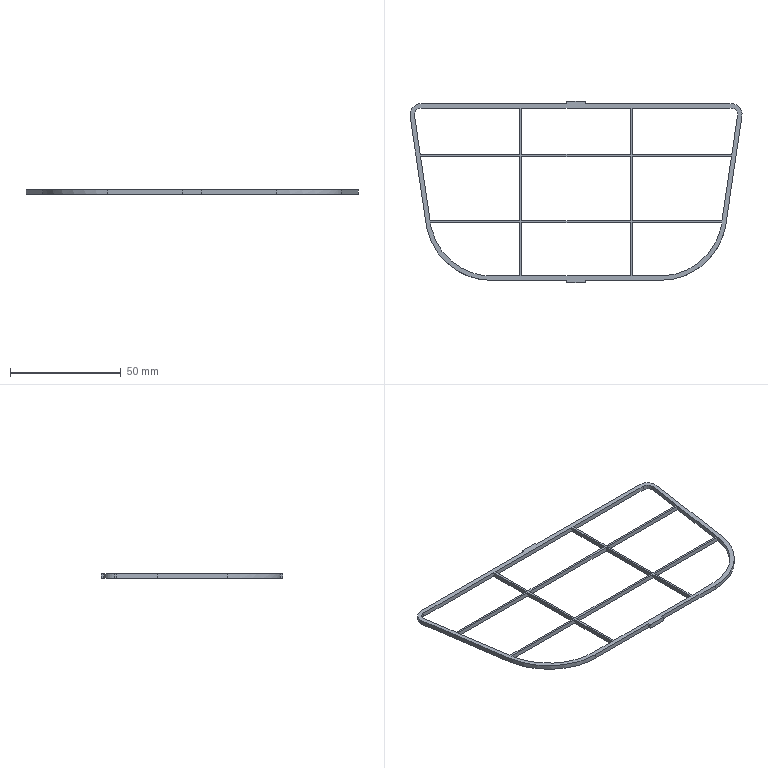Part | SolidWorks | features SplitBody 1 | 1 solid | 61 faces | box 150.242 x 82 x 2 mm | volume 2520 mm3 | plane 51 | cylinder 6 | spline 4 | commonest cylinder face diameters 6 x3 10 x3